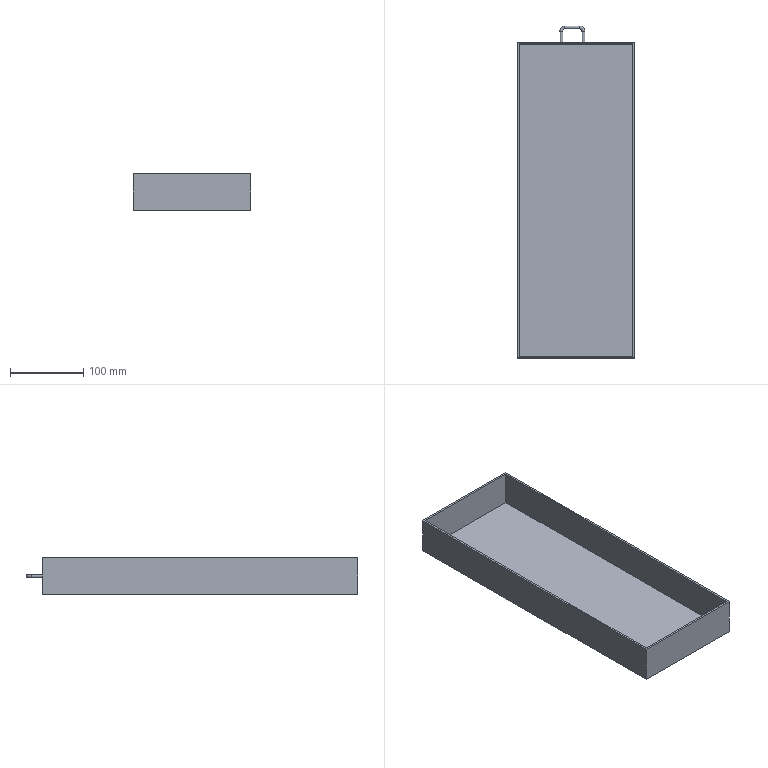Part | NX | features solid 2 | 1 solid | 16 faces | box 160 x 452 x 50 mm | volume 311763 mm3 | plane 11 | cylinder 3 | torus 2 | commonest cylinder face diameters 4 x3
STEP:
#1=CARTESIAN_POINT('',(322.,375.,-348.));
#2=VERTEX_POINT('',#1);
#3=CARTESIAN_POINT('',(322.,375.,-350.));
#4=DIRECTION('',(0.,1.,0.));
#5=DIRECTION('',(0.,0.,1.));
#6=AXIS2_PLACEMENT_3D('',#3,#4,#5);
#7=CIRCLE('',#6,2.);
#8=EDGE_CURVE('',#2,#2,#7,.T.);
#9=ORIENTED_EDGE('',*,*,#8,.F.);
#10=EDGE_LOOP('',(#9));
#11=FACE_BOUND('',#10,.T.);
#12=CARTESIAN_POINT('',(262.,375.,-375.));
#13=VERTEX_POINT('',#12);
#14=CARTESIAN_POINT('',(422.,375.,-375.));
#15=VERTEX_POINT('',#14);
#16=CARTESIAN_POINT('',(262.,375.,-375.));
#17=DIRECTION('',(1.,0.,0.));
#18=VECTOR('',#17,1000.);
#19=LINE('',#16,#18);
#20=EDGE_CURVE('',#13,#15,#19,.T.);
#21=ORIENTED_EDGE('',*,*,#20,.F.);
#22=CARTESIAN_POINT('',(262.,375.,-325.));
#23=VERTEX_POINT('',#22);
#24=CARTESIAN_POINT('',(262.,375.,-325.));
#25=DIRECTION('',(0.,0.,-1.));
#26=VECTOR('',#25,1000.);
#27=LINE('',#24,#26);
#28=EDGE_CURVE('',#23,#13,#27,.T.);
#29=ORIENTED_EDGE('',*,*,#28,.F.);
#30=CARTESIAN_POINT('',(422.,375.,-325.));
#31=VERTEX_POINT('',#30);
#32=CARTESIAN_POINT('',(262.,375.,-325.));
#33=DIRECTION('',(1.,0.,0.));
#34=VECTOR('',#33,1000.);
#35=LINE('',#32,#34);
#36=EDGE_CURVE('',#23,#31,#35,.T.);
#37=ORIENTED_EDGE('',*,*,#36,.T.);
#38=CARTESIAN_POINT('',(422.,375.,-325.));
#39=DIRECTION('',(0.,0.,-1.));
#40=VECTOR('',#39,1000.);
#41=LINE('',#38,#40);
#42=EDGE_CURVE('',#31,#15,#41,.T.);
#43=ORIENTED_EDGE('',*,*,#42,.T.);
#44=EDGE_LOOP('',(#21,#29,#37,#43));
#45=FACE_BOUND('',#44,.T.);
#46=CARTESIAN_POINT('',(352.,375.,-348.));
#47=VERTEX_POINT('',#46);
#48=CARTESIAN_POINT('',(352.,375.,-350.));
#49=DIRECTION('',(0.,1.,0.));
#50=DIRECTION('',(0.,0.,1.));
#51=AXIS2_PLACEMENT_3D('',#48,#49,#50);
#52=CIRCLE('',#51,2.);
#53=EDGE_CURVE('',#47,#47,#52,.T.);
#54=ORIENTED_EDGE('',*,*,#53,.F.);
#55=EDGE_LOOP('',(#54));
#56=FACE_BOUND('',#55,.T.);
#57=CARTESIAN_POINT('',(262.,375.,-325.));
#58=DIRECTION('',(0.,1.,0.));
#59=DIRECTION('',(0.,0.,1.));
#60=AXIS2_PLACEMENT_3D('',#57,#58,#59);
#61=PLANE('',#60);
#62=ADVANCED_FACE('',(#11,#45,#56),#61,.T.);
#63=CARTESIAN_POINT('',(419.5,372.5,-372.5));
#64=VERTEX_POINT('',#63);
#65=CARTESIAN_POINT('',(419.5,-52.5,-372.5));
#66=VERTEX_POINT('',#65);
#67=CARTESIAN_POINT('',(419.5,182.5,-372.5));
#68=DIRECTION('',(0.,-1.,0.));
#69=VECTOR('',#68,1000.);
#70=LINE('',#67,#69);
#71=EDGE_CURVE('',#64,#66,#70,.T.);
#72=ORIENTED_EDGE('',*,*,#71,.F.);
#73=CARTESIAN_POINT('',(264.5,372.5,-372.5));
#74=VERTEX_POINT('',#73);
#75=CARTESIAN_POINT('',(264.5,372.5,-372.5));
#76=DIRECTION('',(1.,0.,0.));
#77=VECTOR('',#76,1000.);
#78=LINE('',#75,#77);
#79=EDGE_CURVE('',#74,#64,#78,.T.);
#80=ORIENTED_EDGE('',*,*,#79,.F.);
#81=CARTESIAN_POINT('',(264.5,-52.5,-372.5));
#82=VERTEX_POINT('',#81);
#83=CARTESIAN_POINT('',(264.5,182.5,-372.5));
#84=DIRECTION('',(0.,1.,0.));
#85=VECTOR('',#84,1000.);
#86=LINE('',#83,#85);
#87=EDGE_CURVE('',#82,#74,#86,.T.);
#88=ORIENTED_EDGE('',*,*,#87,.F.);
#89=CARTESIAN_POINT('',(262.,-52.5,-372.5));
#90=DIRECTION('',(-1.,0.,0.));
#91=VECTOR('',#90,1000.);
#92=LINE('',#89,#91);
#93=EDGE_CURVE('',#66,#82,#92,.T.);
#94=ORIENTED_EDGE('',*,*,#93,.F.);
#95=EDGE_LOOP('',(#72,#80,#88,#94));
#96=FACE_BOUND('',#95,.T.);
#97=CARTESIAN_POINT('',(409.5,182.5,-372.5));
#98=DIRECTION('',(0.,0.,-1.));
#99=DIRECTION('',(-1.,0.,0.));
#100=AXIS2_PLACEMENT_3D('',#97,#98,#99);
#101=PLANE('',#100);
#102=ADVANCED_FACE('',(#96),#101,.F.);
#103=CARTESIAN_POINT('',(422.,-55.,-375.));
#104=VERTEX_POINT('',#103);
#105=CARTESIAN_POINT('',(262.,-55.,-375.));
#106=VERTEX_POINT('',#105);
#107=CARTESIAN_POINT('',(409.5,-55.,-375.));
#108=DIRECTION('',(-1.,0.,0.));
#109=VECTOR('',#108,1000.);
#110=LINE('',#107,#109);
#111=EDGE_CURVE('',#104,#106,#110,.T.);
#112=ORIENTED_EDGE('',*,*,#111,.T.);
#113=CARTESIAN_POINT('',(262.,372.5,-375.));
#114=DIRECTION('',(0.,1.,0.));
#115=VECTOR('',#114,1000.);
#116=LINE('',#113,#115);
#117=EDGE_CURVE('',#106,#13,#116,.T.);
#118=ORIENTED_EDGE('',*,*,#117,.T.);
#119=ORIENTED_EDGE('',*,*,#20,.T.);
#120=CARTESIAN_POINT('',(422.,182.5,-375.));
#121=DIRECTION('',(0.,-1.,0.));
#122=VECTOR('',#121,1000.);
#123=LINE('',#120,#122);
#124=EDGE_CURVE('',#15,#104,#123,.T.);
#125=ORIENTED_EDGE('',*,*,#124,.T.);
#126=EDGE_LOOP('',(#112,#118,#119,#125));
#127=FACE_BOUND('',#126,.T.);
#128=CARTESIAN_POINT('',(409.5,182.5,-375.));
#129=DIRECTION('',(0.,0.,-1.));
#130=DIRECTION('',(-1.,0.,0.));
#131=AXIS2_PLACEMENT_3D('',#128,#129,#130);
#132=PLANE('',#131);
#133=ADVANCED_FACE('',(#127),#132,.T.);
#134=CARTESIAN_POINT('',(419.5,372.5,-325.));
#135=VERTEX_POINT('',#134);
#136=CARTESIAN_POINT('',(419.5,372.5,-325.));
#137=DIRECTION('',(0.,0.,-1.));
#138=VECTOR('',#137,1000.);
#139=LINE('',#136,#138);
#140=EDGE_CURVE('',#135,#64,#139,.T.);
#141=ORIENTED_EDGE('',*,*,#140,.F.);
#142=CARTESIAN_POINT('',(264.5,372.5,-325.));
#143=VERTEX_POINT('',#142);
#144=CARTESIAN_POINT('',(412.,372.5,-325.));
#145=DIRECTION('',(-1.,0.,0.));
#146=VECTOR('',#145,1000.);
#147=LINE('',#144,#146);
#148=EDGE_CURVE('',#135,#143,#147,.T.);
#149=ORIENTED_EDGE('',*,*,#148,.T.);
#150=CARTESIAN_POINT('',(264.5,372.5,-325.));
#151=DIRECTION('',(0.,0.,-1.));
#152=VECTOR('',#151,1000.);
#153=LINE('',#150,#152);
#154=EDGE_CURVE('',#143,#74,#153,.T.);
#155=ORIENTED_EDGE('',*,*,#154,.T.);
#156=ORIENTED_EDGE('',*,*,#79,.T.);
#157=EDGE_LOOP('',(#141,#149,#155,#156));
#158=FACE_BOUND('',#157,.T.);
#159=CARTESIAN_POINT('',(412.,372.5,-325.));
#160=DIRECTION('',(0.,-1.,0.));
#161=DIRECTION('',(0.,0.,-1.));
#162=AXIS2_PLACEMENT_3D('',#159,#160,#161);
#163=PLANE('',#162);
#164=ADVANCED_FACE('',(#158),#163,.T.);
#165=ORIENTED_EDGE('',*,*,#124,.F.);
#166=ORIENTED_EDGE('',*,*,#42,.F.);
#167=CARTESIAN_POINT('',(422.,-55.,-325.));
#168=VERTEX_POINT('',#167);
#169=CARTESIAN_POINT('',(422.,372.5,-325.));
#170=DIRECTION('',(0.,-1.,0.));
#171=VECTOR('',#170,1000.);
#172=LINE('',#169,#171);
#173=EDGE_CURVE('',#31,#168,#172,.T.);
#174=ORIENTED_EDGE('',*,*,#173,.T.);
#175=CARTESIAN_POINT('',(422.,-55.,-325.));
#176=DIRECTION('',(0.,0.,-1.));
#177=VECTOR('',#176,1000.);
#178=LINE('',#175,#177);
#179=EDGE_CURVE('',#168,#104,#178,.T.);
#180=ORIENTED_EDGE('',*,*,#179,.T.);
#181=EDGE_LOOP('',(#165,#166,#174,#180));
#182=FACE_BOUND('',#181,.T.);
#183=CARTESIAN_POINT('',(422.,375.,-325.));
#184=DIRECTION('',(1.,0.,0.));
#185=DIRECTION('',(0.,0.,-1.));
#186=AXIS2_PLACEMENT_3D('',#183,#184,#185);
#187=PLANE('',#186);
#188=ADVANCED_FACE('',(#182),#187,.T.);
#189=ORIENTED_EDGE('',*,*,#117,.F.);
#190=CARTESIAN_POINT('',(262.,-55.,-325.));
#191=VERTEX_POINT('',#190);
#192=CARTESIAN_POINT('',(262.,-55.,-325.));
#193=DIRECTION('',(0.,0.,-1.));
#194=VECTOR('',#193,1000.);
#195=LINE('',#192,#194);
#196=EDGE_CURVE('',#191,#106,#195,.T.);
#197=ORIENTED_EDGE('',*,*,#196,.F.);
#198=CARTESIAN_POINT('',(262.,372.5,-325.));
#199=DIRECTION('',(0.,1.,0.));
#200=VECTOR('',#199,1000.);
#201=LINE('',#198,#200);
#202=EDGE_CURVE('',#191,#23,#201,.T.);
#203=ORIENTED_EDGE('',*,*,#202,.T.);
#204=ORIENTED_EDGE('',*,*,#28,.T.);
#205=EDGE_LOOP('',(#189,#197,#203,#204));
#206=FACE_BOUND('',#205,.T.);
#207=CARTESIAN_POINT('',(262.,372.5,-325.));
#208=DIRECTION('',(-1.,0.,0.));
#209=DIRECTION('',(0.,0.,1.));
#210=AXIS2_PLACEMENT_3D('',#207,#208,#209);
#211=PLANE('',#210);
#212=ADVANCED_FACE('',(#206),#211,.T.);
#213=ORIENTED_EDGE('',*,*,#148,.F.);
#214=CARTESIAN_POINT('',(419.5,-52.5,-325.));
#215=VERTEX_POINT('',#214);
#216=CARTESIAN_POINT('',(419.5,372.5,-325.));
#217=DIRECTION('',(0.,1.,0.));
#218=VECTOR('',#217,1000.);
#219=LINE('',#216,#218);
#220=EDGE_CURVE('',#215,#135,#219,.T.);
#221=ORIENTED_EDGE('',*,*,#220,.F.);
#222=CARTESIAN_POINT('',(264.5,-52.5,-325.));
#223=VERTEX_POINT('',#222);
#224=CARTESIAN_POINT('',(412.,-52.5,-325.));
#225=DIRECTION('',(1.,0.,0.));
#226=VECTOR('',#225,1000.);
#227=LINE('',#224,#226);
#228=EDGE_CURVE('',#223,#215,#227,.T.);
#229=ORIENTED_EDGE('',*,*,#228,.F.);
#230=CARTESIAN_POINT('',(264.5,372.5,-325.));
#231=DIRECTION('',(0.,-1.,0.));
#232=VECTOR('',#231,1000.);
#233=LINE('',#230,#232);
#234=EDGE_CURVE('',#143,#223,#233,.T.);
#235=ORIENTED_EDGE('',*,*,#234,.F.);
#236=EDGE_LOOP('',(#213,#221,#229,#235));
#237=FACE_BOUND('',#236,.T.);
#238=ORIENTED_EDGE('',*,*,#173,.F.);
#239=ORIENTED_EDGE('',*,*,#36,.F.);
#240=ORIENTED_EDGE('',*,*,#202,.F.);
#241=CARTESIAN_POINT('',(412.,-55.,-325.));
#242=DIRECTION('',(-1.,0.,0.));
#243=VECTOR('',#242,1000.);
#244=LINE('',#241,#243);
#245=EDGE_CURVE('',#168,#191,#244,.T.);
#246=ORIENTED_EDGE('',*,*,#245,.F.);
#247=EDGE_LOOP('',(#238,#239,#240,#246));
#248=FACE_BOUND('',#247,.T.);
#249=CARTESIAN_POINT('',(412.,372.5,-325.));
#250=DIRECTION('',(0.,0.,-1.));
#251=DIRECTION('',(-1.,0.,0.));
#252=AXIS2_PLACEMENT_3D('',#249,#250,#251);
#253=PLANE('',#252);
#254=ADVANCED_FACE('',(#237,#248),#253,.F.);
#255=CARTESIAN_POINT('',(419.5,-52.5,-325.));
#256=DIRECTION('',(0.,0.,-1.));
#257=VECTOR('',#256,1000.);
#258=LINE('',#255,#257);
#259=EDGE_CURVE('',#215,#66,#258,.T.);
#260=ORIENTED_EDGE('',*,*,#259,.T.);
#261=ORIENTED_EDGE('',*,*,#93,.T.);
#262=CARTESIAN_POINT('',(264.5,-52.5,-325.));
#263=DIRECTION('',(0.,0.,-1.));
#264=VECTOR('',#263,1000.);
#265=LINE('',#262,#264);
#266=EDGE_CURVE('',#223,#82,#265,.T.);
#267=ORIENTED_EDGE('',*,*,#266,.F.);
#268=ORIENTED_EDGE('',*,*,#228,.T.);
#269=EDGE_LOOP('',(#260,#261,#267,#268));
#270=FACE_BOUND('',#269,.T.);
#271=CARTESIAN_POINT('',(262.,-52.5,-325.));
#272=DIRECTION('',(0.,1.,0.));
#273=DIRECTION('',(0.,0.,1.));
#274=AXIS2_PLACEMENT_3D('',#271,#272,#273);
#275=PLANE('',#274);
#276=ADVANCED_FACE('',(#270),#275,.T.);
#277=ORIENTED_EDGE('',*,*,#111,.F.);
#278=ORIENTED_EDGE('',*,*,#179,.F.);
#279=ORIENTED_EDGE('',*,*,#245,.T.);
#280=ORIENTED_EDGE('',*,*,#196,.T.);
#281=EDGE_LOOP('',(#277,#278,#279,#280));
#282=FACE_BOUND('',#281,.T.);
#283=CARTESIAN_POINT('',(412.,-55.,-325.));
#284=DIRECTION('',(0.,-1.,0.));
#285=DIRECTION('',(0.,0.,-1.));
#286=AXIS2_PLACEMENT_3D('',#283,#284,#285);
#287=PLANE('',#286);
#288=ADVANCED_FACE('',(#282),#287,.T.);
#289=ORIENTED_EDGE('',*,*,#87,.T.);
#290=ORIENTED_EDGE('',*,*,#154,.F.);
#291=ORIENTED_EDGE('',*,*,#234,.T.);
#292=ORIENTED_EDGE('',*,*,#266,.T.);
#293=EDGE_LOOP('',(#289,#290,#291,#292));
#294=FACE_BOUND('',#293,.T.);
#295=CARTESIAN_POINT('',(264.5,372.5,-325.));
#296=DIRECTION('',(1.,0.,0.));
#297=DIRECTION('',(0.,0.,-1.));
#298=AXIS2_PLACEMENT_3D('',#295,#296,#297);
#299=PLANE('',#298);
#300=ADVANCED_FACE('',(#294),#299,.T.);
#301=ORIENTED_EDGE('',*,*,#71,.T.);
#302=ORIENTED_EDGE('',*,*,#259,.F.);
#303=ORIENTED_EDGE('',*,*,#220,.T.);
#304=ORIENTED_EDGE('',*,*,#140,.T.);
#305=EDGE_LOOP('',(#301,#302,#303,#304));
#306=FACE_BOUND('',#305,.T.);
#307=CARTESIAN_POINT('',(419.5,182.5,-325.));
#308=DIRECTION('',(-1.,0.,0.));
#309=DIRECTION('',(0.,0.,1.));
#310=AXIS2_PLACEMENT_3D('',#307,#308,#309);
#311=PLANE('',#310);
#312=ADVANCED_FACE('',(#306),#311,.T.);
#313=CARTESIAN_POINT('',(322.,390.,-348.));
#314=VERTEX_POINT('',#313);
#315=CARTESIAN_POINT('',(322.,390.,-350.));
#316=DIRECTION('',(0.,-1.,0.));
#317=DIRECTION('',(0.,0.,1.));
#318=AXIS2_PLACEMENT_3D('',#315,#316,#317);
#319=CIRCLE('',#318,2.);
#320=EDGE_CURVE('',#314,#314,#319,.T.);
#321=ORIENTED_EDGE('',*,*,#320,.T.);
#322=EDGE_LOOP('',(#321));
#323=FACE_BOUND('',#322,.T.);
#324=ORIENTED_EDGE('',*,*,#8,.T.);
#325=EDGE_LOOP('',(#324));
#326=FACE_BOUND('',#325,.T.);
#327=CARTESIAN_POINT('',(322.,390.,-350.));
#328=DIRECTION('',(0.,-1.,0.));
#329=DIRECTION('',(0.,0.,-1.));
#330=AXIS2_PLACEMENT_3D('',#327,#328,#329);
#331=CYLINDRICAL_SURFACE('',#330,2.);
#332=ADVANCED_FACE('',(#323,#326),#331,.T.);
#333=CARTESIAN_POINT('',(327.,395.,-348.));
#334=VERTEX_POINT('',#333);
#335=CARTESIAN_POINT('',(327.,395.,-350.));
#336=DIRECTION('',(-1.,0.,0.));
#337=DIRECTION('',(0.,0.,1.));
#338=AXIS2_PLACEMENT_3D('',#335,#336,#337);
#339=CIRCLE('',#338,2.);
#340=EDGE_CURVE('',#334,#334,#339,.T.);
#341=ORIENTED_EDGE('',*,*,#340,.T.);
#342=EDGE_LOOP('',(#341));
#343=FACE_BOUND('',#342,.T.);
#344=ORIENTED_EDGE('',*,*,#320,.F.);
#345=EDGE_LOOP('',(#344));
#346=FACE_BOUND('',#345,.T.);
#347=CARTESIAN_POINT('',(327.,390.,-350.));
#348=DIRECTION('',(0.,0.,1.));
#349=DIRECTION('',(1.,0.,0.));
#350=AXIS2_PLACEMENT_3D('',#347,#348,#349);
#351=TOROIDAL_SURFACE('',#350,5.,2.);
#352=ADVANCED_FACE('',(#343,#346),#351,.T.);
#353=CARTESIAN_POINT('',(347.,395.,-348.));
#354=VERTEX_POINT('',#353);
#355=CARTESIAN_POINT('',(347.,395.,-350.));
#356=DIRECTION('',(-1.,0.,0.));
#357=DIRECTION('',(0.,0.,1.));
#358=AXIS2_PLACEMENT_3D('',#355,#356,#357);
#359=CIRCLE('',#358,2.);
#360=EDGE_CURVE('',#354,#354,#359,.T.);
#361=ORIENTED_EDGE('',*,*,#360,.T.);
#362=EDGE_LOOP('',(#361));
#363=FACE_BOUND('',#362,.T.);
#364=ORIENTED_EDGE('',*,*,#340,.F.);
#365=EDGE_LOOP('',(#364));
#366=FACE_BOUND('',#365,.T.);
#367=CARTESIAN_POINT('',(347.,395.,-350.));
#368=DIRECTION('',(-1.,0.,0.));
#369=DIRECTION('',(0.,0.,1.));
#370=AXIS2_PLACEMENT_3D('',#367,#368,#369);
#371=CYLINDRICAL_SURFACE('',#370,2.);
#372=ADVANCED_FACE('',(#363,#366),#371,.T.);
#373=CARTESIAN_POINT('',(352.,390.,-348.));
#374=VERTEX_POINT('',#373);
#375=CARTESIAN_POINT('',(352.,390.,-350.));
#376=DIRECTION('',(0.,1.,0.));
#377=DIRECTION('',(0.,0.,1.));
#378=AXIS2_PLACEMENT_3D('',#375,#376,#377);
#379=CIRCLE('',#378,2.);
#380=EDGE_CURVE('',#374,#374,#379,.T.);
#381=ORIENTED_EDGE('',*,*,#380,.T.);
#382=EDGE_LOOP('',(#381));
#383=FACE_BOUND('',#382,.T.);
#384=ORIENTED_EDGE('',*,*,#360,.F.);
#385=EDGE_LOOP('',(#384));
#386=FACE_BOUND('',#385,.T.);
#387=CARTESIAN_POINT('',(347.,390.,-350.));
#388=DIRECTION('',(0.,0.,1.));
#389=DIRECTION('',(1.,0.,0.));
#390=AXIS2_PLACEMENT_3D('',#387,#388,#389);
#391=TOROIDAL_SURFACE('',#390,5.,2.);
#392=ADVANCED_FACE('',(#383,#386),#391,.T.);
#393=ORIENTED_EDGE('',*,*,#380,.F.);
#394=EDGE_LOOP('',(#393));
#395=FACE_BOUND('',#394,.T.);
#396=ORIENTED_EDGE('',*,*,#53,.T.);
#397=EDGE_LOOP('',(#396));
#398=FACE_BOUND('',#397,.T.);
#399=CARTESIAN_POINT('',(352.,390.,-350.));
#400=DIRECTION('',(0.,-1.,0.));
#401=DIRECTION('',(0.,0.,-1.));
#402=AXIS2_PLACEMENT_3D('',#399,#400,#401);
#403=CYLINDRICAL_SURFACE('',#402,2.);
#404=ADVANCED_FACE('',(#395,#398),#403,.T.);
#405=CLOSED_SHELL('',(#62,#102,#133,#164,#188,#212,#254,#276,#288,#300,#312,#332,#352,#372,#392,#404));
#406=MANIFOLD_SOLID_BREP('',#405);
#407=(LENGTH_UNIT()NAMED_UNIT(*)SI_UNIT(.MILLI.,.METRE.));
#408=UNCERTAINTY_MEASURE_WITH_UNIT(LENGTH_MEASURE(0.00001),#407,'','');
#409=(NAMED_UNIT(*)PLANE_ANGLE_UNIT()SI_UNIT($,.RADIAN.));
#410=(NAMED_UNIT(*)SI_UNIT($,.STERADIAN.)SOLID_ANGLE_UNIT());
#411=(GEOMETRIC_REPRESENTATION_CONTEXT(3)GLOBAL_UNCERTAINTY_ASSIGNED_CONTEXT((#408))GLOBAL_UNIT_ASSIGNED_CONTEXT((#407,#409,#410))REPRESENTATION_CONTEXT('',''));
#412=ADVANCED_BREP_SHAPE_REPRESENTATION('',(#406),#411);